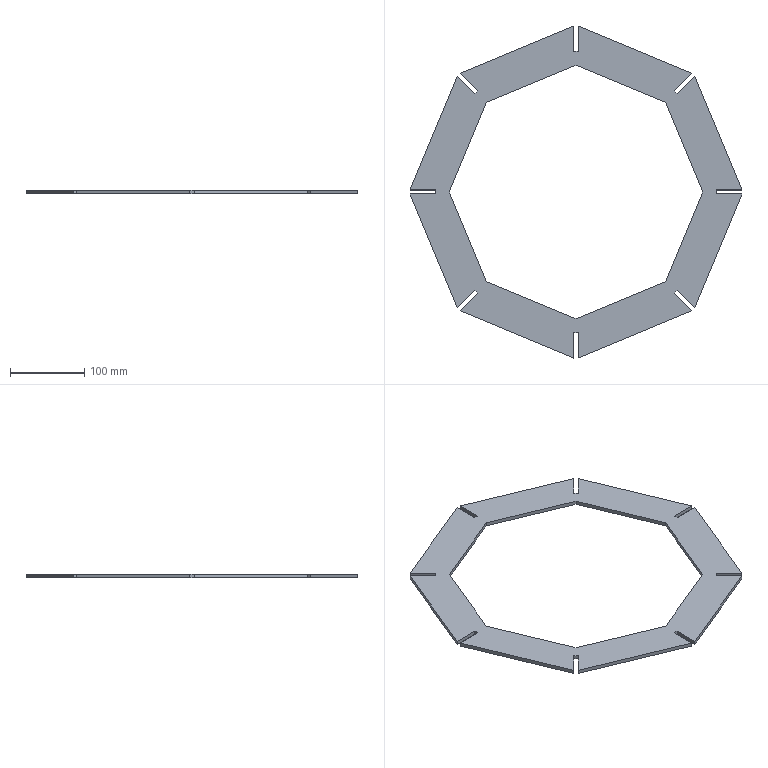Part | SolidWorks | features ICE 2, Extrusion 1 | 1 solid | 42 faces | box 447.763 x 447.763 x 5 mm | volume 295555 mm3 | plane 42
STEP:
#1=CARTESIAN_POINT('',(-2.7,223.882,0.));
#2=VERTEX_POINT('',#1);
#3=CARTESIAN_POINT('',(-156.399,160.217,0.));
#4=VERTEX_POINT('',#3);
#5=CARTESIAN_POINT('',(0.,225.,0.));
#6=DIRECTION('',(-0.9239,-0.3827,0.));
#7=VECTOR('',#6,1000.);
#8=LINE('',#5,#7);
#9=EDGE_CURVE('',#2,#4,#8,.T.);
#10=ORIENTED_EDGE('',*,*,#9,.T.);
#11=CARTESIAN_POINT('',(-156.399,160.217,5.));
#12=VERTEX_POINT('',#11);
#13=CARTESIAN_POINT('',(-156.399,160.217,5.));
#14=DIRECTION('',(0.,0.,1.));
#15=VECTOR('',#14,1000.);
#16=LINE('',#13,#15);
#17=EDGE_CURVE('',#4,#12,#16,.T.);
#18=ORIENTED_EDGE('',*,*,#17,.T.);
#19=CARTESIAN_POINT('',(-2.7,223.882,5.));
#20=VERTEX_POINT('',#19);
#21=CARTESIAN_POINT('',(0.,225.,5.));
#22=DIRECTION('',(-0.9239,-0.3827,0.));
#23=VECTOR('',#22,1000.);
#24=LINE('',#21,#23);
#25=EDGE_CURVE('',#20,#12,#24,.T.);
#26=ORIENTED_EDGE('',*,*,#25,.F.);
#27=CARTESIAN_POINT('',(-2.7,223.882,5.));
#28=DIRECTION('',(0.,0.,-1.));
#29=VECTOR('',#28,1000.);
#30=LINE('',#27,#29);
#31=EDGE_CURVE('',#20,#2,#30,.T.);
#32=ORIENTED_EDGE('',*,*,#31,.T.);
#33=EDGE_LOOP('',(#10,#18,#26,#32));
#34=FACE_OUTER_BOUND('',#33,.T.);
#35=CARTESIAN_POINT('',(0.,225.,5.));
#36=DIRECTION('',(0.3827,-0.9239,0.));
#37=DIRECTION('',(0.9239,0.3827,0.));
#38=AXIS2_PLACEMENT_3D('',#35,#36,#37);
#39=PLANE('',#38);
#40=ADVANCED_FACE('',(#34),#39,.F.);
#41=CARTESIAN_POINT('',(-160.217,156.399,0.));
#42=VERTEX_POINT('',#41);
#43=CARTESIAN_POINT('',(-223.882,2.7,0.));
#44=VERTEX_POINT('',#43);
#45=CARTESIAN_POINT('',(-159.099,159.099,0.));
#46=DIRECTION('',(-0.3827,-0.9239,0.));
#47=VECTOR('',#46,1000.);
#48=LINE('',#45,#47);
#49=EDGE_CURVE('',#42,#44,#48,.T.);
#50=ORIENTED_EDGE('',*,*,#49,.T.);
#51=CARTESIAN_POINT('',(-223.882,2.7,5.));
#52=VERTEX_POINT('',#51);
#53=CARTESIAN_POINT('',(-223.882,2.7,5.));
#54=DIRECTION('',(0.,0.,1.));
#55=VECTOR('',#54,1000.);
#56=LINE('',#53,#55);
#57=EDGE_CURVE('',#44,#52,#56,.T.);
#58=ORIENTED_EDGE('',*,*,#57,.T.);
#59=CARTESIAN_POINT('',(-160.217,156.399,5.));
#60=VERTEX_POINT('',#59);
#61=CARTESIAN_POINT('',(-159.099,159.099,5.));
#62=DIRECTION('',(-0.3827,-0.9239,0.));
#63=VECTOR('',#62,1000.);
#64=LINE('',#61,#63);
#65=EDGE_CURVE('',#60,#52,#64,.T.);
#66=ORIENTED_EDGE('',*,*,#65,.F.);
#67=CARTESIAN_POINT('',(-160.217,156.399,5.));
#68=DIRECTION('',(0.,0.,-1.));
#69=VECTOR('',#68,1000.);
#70=LINE('',#67,#69);
#71=EDGE_CURVE('',#60,#42,#70,.T.);
#72=ORIENTED_EDGE('',*,*,#71,.T.);
#73=EDGE_LOOP('',(#50,#58,#66,#72));
#74=FACE_OUTER_BOUND('',#73,.T.);
#75=CARTESIAN_POINT('',(-159.099,159.099,5.));
#76=DIRECTION('',(0.9239,-0.3827,0.));
#77=DIRECTION('',(0.3827,0.9239,0.));
#78=AXIS2_PLACEMENT_3D('',#75,#76,#77);
#79=PLANE('',#78);
#80=ADVANCED_FACE('',(#74),#79,.F.);
#81=CARTESIAN_POINT('',(-223.882,-2.7,0.));
#82=VERTEX_POINT('',#81);
#83=CARTESIAN_POINT('',(-160.217,-156.399,0.));
#84=VERTEX_POINT('',#83);
#85=CARTESIAN_POINT('',(-225.,0.,0.));
#86=DIRECTION('',(0.3827,-0.9239,0.));
#87=VECTOR('',#86,1000.);
#88=LINE('',#85,#87);
#89=EDGE_CURVE('',#82,#84,#88,.T.);
#90=ORIENTED_EDGE('',*,*,#89,.T.);
#91=CARTESIAN_POINT('',(-160.217,-156.399,5.));
#92=VERTEX_POINT('',#91);
#93=CARTESIAN_POINT('',(-160.217,-156.399,5.));
#94=DIRECTION('',(0.,0.,1.));
#95=VECTOR('',#94,1000.);
#96=LINE('',#93,#95);
#97=EDGE_CURVE('',#84,#92,#96,.T.);
#98=ORIENTED_EDGE('',*,*,#97,.T.);
#99=CARTESIAN_POINT('',(-223.882,-2.7,5.));
#100=VERTEX_POINT('',#99);
#101=CARTESIAN_POINT('',(-225.,0.,5.));
#102=DIRECTION('',(0.3827,-0.9239,0.));
#103=VECTOR('',#102,1000.);
#104=LINE('',#101,#103);
#105=EDGE_CURVE('',#100,#92,#104,.T.);
#106=ORIENTED_EDGE('',*,*,#105,.F.);
#107=CARTESIAN_POINT('',(-223.882,-2.7,5.));
#108=DIRECTION('',(0.,0.,-1.));
#109=VECTOR('',#108,1000.);
#110=LINE('',#107,#109);
#111=EDGE_CURVE('',#100,#82,#110,.T.);
#112=ORIENTED_EDGE('',*,*,#111,.T.);
#113=EDGE_LOOP('',(#90,#98,#106,#112));
#114=FACE_OUTER_BOUND('',#113,.T.);
#115=CARTESIAN_POINT('',(-225.,0.,5.));
#116=DIRECTION('',(0.9239,0.3827,0.));
#117=DIRECTION('',(-0.3827,0.9239,0.));
#118=AXIS2_PLACEMENT_3D('',#115,#116,#117);
#119=PLANE('',#118);
#120=ADVANCED_FACE('',(#114),#119,.F.);
#121=CARTESIAN_POINT('',(-156.399,-160.217,0.));
#122=VERTEX_POINT('',#121);
#123=CARTESIAN_POINT('',(-2.7,-223.882,0.));
#124=VERTEX_POINT('',#123);
#125=CARTESIAN_POINT('',(-159.099,-159.099,0.));
#126=DIRECTION('',(0.9239,-0.3827,0.));
#127=VECTOR('',#126,1000.);
#128=LINE('',#125,#127);
#129=EDGE_CURVE('',#122,#124,#128,.T.);
#130=ORIENTED_EDGE('',*,*,#129,.T.);
#131=CARTESIAN_POINT('',(-2.7,-223.882,5.));
#132=VERTEX_POINT('',#131);
#133=CARTESIAN_POINT('',(-2.7,-223.882,5.));
#134=DIRECTION('',(0.,0.,1.));
#135=VECTOR('',#134,1000.);
#136=LINE('',#133,#135);
#137=EDGE_CURVE('',#124,#132,#136,.T.);
#138=ORIENTED_EDGE('',*,*,#137,.T.);
#139=CARTESIAN_POINT('',(-156.399,-160.217,5.));
#140=VERTEX_POINT('',#139);
#141=CARTESIAN_POINT('',(-159.099,-159.099,5.));
#142=DIRECTION('',(0.9239,-0.3827,0.));
#143=VECTOR('',#142,1000.);
#144=LINE('',#141,#143);
#145=EDGE_CURVE('',#140,#132,#144,.T.);
#146=ORIENTED_EDGE('',*,*,#145,.F.);
#147=CARTESIAN_POINT('',(-156.399,-160.217,5.));
#148=DIRECTION('',(0.,0.,-1.));
#149=VECTOR('',#148,1000.);
#150=LINE('',#147,#149);
#151=EDGE_CURVE('',#140,#122,#150,.T.);
#152=ORIENTED_EDGE('',*,*,#151,.T.);
#153=EDGE_LOOP('',(#130,#138,#146,#152));
#154=FACE_OUTER_BOUND('',#153,.T.);
#155=CARTESIAN_POINT('',(-159.099,-159.099,5.));
#156=DIRECTION('',(0.3827,0.9239,0.));
#157=DIRECTION('',(-0.9239,0.3827,0.));
#158=AXIS2_PLACEMENT_3D('',#155,#156,#157);
#159=PLANE('',#158);
#160=ADVANCED_FACE('',(#154),#159,.F.);
#161=CARTESIAN_POINT('',(2.7,-223.882,0.));
#162=VERTEX_POINT('',#161);
#163=CARTESIAN_POINT('',(156.399,-160.217,0.));
#164=VERTEX_POINT('',#163);
#165=CARTESIAN_POINT('',(0.,-225.,0.));
#166=DIRECTION('',(0.9239,0.3827,0.));
#167=VECTOR('',#166,1000.);
#168=LINE('',#165,#167);
#169=EDGE_CURVE('',#162,#164,#168,.T.);
#170=ORIENTED_EDGE('',*,*,#169,.T.);
#171=CARTESIAN_POINT('',(156.399,-160.217,5.));
#172=VERTEX_POINT('',#171);
#173=CARTESIAN_POINT('',(156.399,-160.217,5.));
#174=DIRECTION('',(0.,0.,1.));
#175=VECTOR('',#174,1000.);
#176=LINE('',#173,#175);
#177=EDGE_CURVE('',#164,#172,#176,.T.);
#178=ORIENTED_EDGE('',*,*,#177,.T.);
#179=CARTESIAN_POINT('',(2.7,-223.882,5.));
#180=VERTEX_POINT('',#179);
#181=CARTESIAN_POINT('',(0.,-225.,5.));
#182=DIRECTION('',(0.9239,0.3827,0.));
#183=VECTOR('',#182,1000.);
#184=LINE('',#181,#183);
#185=EDGE_CURVE('',#180,#172,#184,.T.);
#186=ORIENTED_EDGE('',*,*,#185,.F.);
#187=CARTESIAN_POINT('',(2.7,-223.882,5.));
#188=DIRECTION('',(0.,0.,-1.));
#189=VECTOR('',#188,1000.);
#190=LINE('',#187,#189);
#191=EDGE_CURVE('',#180,#162,#190,.T.);
#192=ORIENTED_EDGE('',*,*,#191,.T.);
#193=EDGE_LOOP('',(#170,#178,#186,#192));
#194=FACE_OUTER_BOUND('',#193,.T.);
#195=CARTESIAN_POINT('',(0.,-225.,5.));
#196=DIRECTION('',(-0.3827,0.9239,0.));
#197=DIRECTION('',(-0.9239,-0.3827,0.));
#198=AXIS2_PLACEMENT_3D('',#195,#196,#197);
#199=PLANE('',#198);
#200=ADVANCED_FACE('',(#194),#199,.F.);
#201=CARTESIAN_POINT('',(160.217,-156.399,0.));
#202=VERTEX_POINT('',#201);
#203=CARTESIAN_POINT('',(223.882,-2.7,0.));
#204=VERTEX_POINT('',#203);
#205=CARTESIAN_POINT('',(159.099,-159.099,0.));
#206=DIRECTION('',(0.3827,0.9239,0.));
#207=VECTOR('',#206,1000.);
#208=LINE('',#205,#207);
#209=EDGE_CURVE('',#202,#204,#208,.T.);
#210=ORIENTED_EDGE('',*,*,#209,.T.);
#211=CARTESIAN_POINT('',(223.882,-2.7,5.));
#212=VERTEX_POINT('',#211);
#213=CARTESIAN_POINT('',(223.882,-2.7,5.));
#214=DIRECTION('',(0.,0.,1.));
#215=VECTOR('',#214,1000.);
#216=LINE('',#213,#215);
#217=EDGE_CURVE('',#204,#212,#216,.T.);
#218=ORIENTED_EDGE('',*,*,#217,.T.);
#219=CARTESIAN_POINT('',(160.217,-156.399,5.));
#220=VERTEX_POINT('',#219);
#221=CARTESIAN_POINT('',(159.099,-159.099,5.));
#222=DIRECTION('',(0.3827,0.9239,0.));
#223=VECTOR('',#222,1000.);
#224=LINE('',#221,#223);
#225=EDGE_CURVE('',#220,#212,#224,.T.);
#226=ORIENTED_EDGE('',*,*,#225,.F.);
#227=CARTESIAN_POINT('',(160.217,-156.399,5.));
#228=DIRECTION('',(0.,0.,-1.));
#229=VECTOR('',#228,1000.);
#230=LINE('',#227,#229);
#231=EDGE_CURVE('',#220,#202,#230,.T.);
#232=ORIENTED_EDGE('',*,*,#231,.T.);
#233=EDGE_LOOP('',(#210,#218,#226,#232));
#234=FACE_OUTER_BOUND('',#233,.T.);
#235=CARTESIAN_POINT('',(159.099,-159.099,5.));
#236=DIRECTION('',(-0.9239,0.3827,0.));
#237=DIRECTION('',(-0.3827,-0.9239,0.));
#238=AXIS2_PLACEMENT_3D('',#235,#236,#237);
#239=PLANE('',#238);
#240=ADVANCED_FACE('',(#234),#239,.F.);
#241=CARTESIAN_POINT('',(223.882,2.7,5.));
#242=VERTEX_POINT('',#241);
#243=CARTESIAN_POINT('',(160.217,156.399,5.));
#244=VERTEX_POINT('',#243);
#245=CARTESIAN_POINT('',(225.,0.,5.));
#246=DIRECTION('',(-0.3827,0.9239,0.));
#247=VECTOR('',#246,1000.);
#248=LINE('',#245,#247);
#249=EDGE_CURVE('',#242,#244,#248,.T.);
#250=ORIENTED_EDGE('',*,*,#249,.F.);
#251=CARTESIAN_POINT('',(223.882,2.7,0.));
#252=VERTEX_POINT('',#251);
#253=CARTESIAN_POINT('',(223.882,2.7,5.));
#254=DIRECTION('',(0.,0.,-1.));
#255=VECTOR('',#254,1000.);
#256=LINE('',#253,#255);
#257=EDGE_CURVE('',#242,#252,#256,.T.);
#258=ORIENTED_EDGE('',*,*,#257,.T.);
#259=CARTESIAN_POINT('',(160.217,156.399,0.));
#260=VERTEX_POINT('',#259);
#261=CARTESIAN_POINT('',(225.,0.,0.));
#262=DIRECTION('',(-0.3827,0.9239,0.));
#263=VECTOR('',#262,1000.);
#264=LINE('',#261,#263);
#265=EDGE_CURVE('',#252,#260,#264,.T.);
#266=ORIENTED_EDGE('',*,*,#265,.T.);
#267=CARTESIAN_POINT('',(160.217,156.399,5.));
#268=DIRECTION('',(0.,0.,1.));
#269=VECTOR('',#268,1000.);
#270=LINE('',#267,#269);
#271=EDGE_CURVE('',#260,#244,#270,.T.);
#272=ORIENTED_EDGE('',*,*,#271,.T.);
#273=EDGE_LOOP('',(#250,#258,#266,#272));
#274=FACE_OUTER_BOUND('',#273,.T.);
#275=CARTESIAN_POINT('',(225.,0.,5.));
#276=DIRECTION('',(-0.9239,-0.3827,0.));
#277=DIRECTION('',(0.3827,-0.9239,0.));
#278=AXIS2_PLACEMENT_3D('',#275,#276,#277);
#279=PLANE('',#278);
#280=ADVANCED_FACE('',(#274),#279,.F.);
#281=CARTESIAN_POINT('',(156.399,160.217,0.));
#282=VERTEX_POINT('',#281);
#283=CARTESIAN_POINT('',(2.7,223.882,0.));
#284=VERTEX_POINT('',#283);
#285=CARTESIAN_POINT('',(159.099,159.099,0.));
#286=DIRECTION('',(-0.9239,0.3827,0.));
#287=VECTOR('',#286,1000.);
#288=LINE('',#285,#287);
#289=EDGE_CURVE('',#282,#284,#288,.T.);
#290=ORIENTED_EDGE('',*,*,#289,.T.);
#291=CARTESIAN_POINT('',(2.7,223.882,5.));
#292=VERTEX_POINT('',#291);
#293=CARTESIAN_POINT('',(2.7,223.882,5.));
#294=DIRECTION('',(0.,0.,1.));
#295=VECTOR('',#294,1000.);
#296=LINE('',#293,#295);
#297=EDGE_CURVE('',#284,#292,#296,.T.);
#298=ORIENTED_EDGE('',*,*,#297,.T.);
#299=CARTESIAN_POINT('',(156.399,160.217,5.));
#300=VERTEX_POINT('',#299);
#301=CARTESIAN_POINT('',(159.099,159.099,5.));
#302=DIRECTION('',(-0.9239,0.3827,0.));
#303=VECTOR('',#302,1000.);
#304=LINE('',#301,#303);
#305=EDGE_CURVE('',#300,#292,#304,.T.);
#306=ORIENTED_EDGE('',*,*,#305,.F.);
#307=CARTESIAN_POINT('',(156.399,160.217,5.));
#308=DIRECTION('',(0.,0.,-1.));
#309=VECTOR('',#308,1000.);
#310=LINE('',#307,#309);
#311=EDGE_CURVE('',#300,#282,#310,.T.);
#312=ORIENTED_EDGE('',*,*,#311,.T.);
#313=EDGE_LOOP('',(#290,#298,#306,#312));
#314=FACE_OUTER_BOUND('',#313,.T.);
#315=CARTESIAN_POINT('',(159.099,159.099,5.));
#316=DIRECTION('',(-0.3827,-0.9239,0.));
#317=DIRECTION('',(0.9239,-0.3827,0.));
#318=AXIS2_PLACEMENT_3D('',#315,#316,#317);
#319=PLANE('',#318);
#320=ADVANCED_FACE('',(#314),#319,.F.);
#321=CARTESIAN_POINT('',(190.,2.7,5.));
#322=VERTEX_POINT('',#321);
#323=CARTESIAN_POINT('',(260.,2.7,5.));
#324=DIRECTION('',(-1.,0.,0.));
#325=VECTOR('',#324,1000.);
#326=LINE('',#323,#325);
#327=EDGE_CURVE('',#242,#322,#326,.T.);
#328=ORIENTED_EDGE('',*,*,#327,.F.);
#329=ORIENTED_EDGE('',*,*,#249,.T.);
#330=CARTESIAN_POINT('',(136.259,132.441,5.));
#331=VERTEX_POINT('',#330);
#332=CARTESIAN_POINT('',(185.757,181.939,5.));
#333=DIRECTION('',(0.7071,0.7071,0.));
#334=VECTOR('',#333,1000.);
#335=LINE('',#332,#334);
#336=EDGE_CURVE('',#331,#244,#335,.T.);
#337=ORIENTED_EDGE('',*,*,#336,.F.);
#338=CARTESIAN_POINT('',(132.441,136.259,5.));
#339=VERTEX_POINT('',#338);
#340=CARTESIAN_POINT('',(136.259,132.441,5.));
#341=DIRECTION('',(0.7071,-0.7071,0.));
#342=VECTOR('',#341,1000.);
#343=LINE('',#340,#342);
#344=EDGE_CURVE('',#339,#331,#343,.T.);
#345=ORIENTED_EDGE('',*,*,#344,.F.);
#346=CARTESIAN_POINT('',(181.939,185.757,5.));
#347=DIRECTION('',(-0.7071,-0.7071,0.));
#348=VECTOR('',#347,1000.);
#349=LINE('',#346,#348);
#350=EDGE_CURVE('',#300,#339,#349,.T.);
#351=ORIENTED_EDGE('',*,*,#350,.F.);
#352=ORIENTED_EDGE('',*,*,#305,.T.);
#353=CARTESIAN_POINT('',(2.7,190.,5.));
#354=VERTEX_POINT('',#353);
#355=CARTESIAN_POINT('',(2.7,260.,5.));
#356=DIRECTION('',(0.,1.,0.));
#357=VECTOR('',#356,1000.);
#358=LINE('',#355,#357);
#359=EDGE_CURVE('',#354,#292,#358,.T.);
#360=ORIENTED_EDGE('',*,*,#359,.F.);
#361=CARTESIAN_POINT('',(-2.7,190.,5.));
#362=VERTEX_POINT('',#361);
#363=CARTESIAN_POINT('',(2.7,190.,5.));
#364=DIRECTION('',(1.,0.,0.));
#365=VECTOR('',#364,1000.);
#366=LINE('',#363,#365);
#367=EDGE_CURVE('',#362,#354,#366,.T.);
#368=ORIENTED_EDGE('',*,*,#367,.F.);
#369=CARTESIAN_POINT('',(-2.7,260.,5.));
#370=DIRECTION('',(0.,-1.,0.));
#371=VECTOR('',#370,1000.);
#372=LINE('',#369,#371);
#373=EDGE_CURVE('',#20,#362,#372,.T.);
#374=ORIENTED_EDGE('',*,*,#373,.F.);
#375=ORIENTED_EDGE('',*,*,#25,.T.);
#376=CARTESIAN_POINT('',(-132.441,136.259,5.));
#377=VERTEX_POINT('',#376);
#378=CARTESIAN_POINT('',(-181.939,185.757,5.));
#379=DIRECTION('',(-0.7071,0.7071,0.));
#380=VECTOR('',#379,1000.);
#381=LINE('',#378,#380);
#382=EDGE_CURVE('',#377,#12,#381,.T.);
#383=ORIENTED_EDGE('',*,*,#382,.F.);
#384=CARTESIAN_POINT('',(-136.259,132.441,5.));
#385=VERTEX_POINT('',#384);
#386=CARTESIAN_POINT('',(-132.441,136.259,5.));
#387=DIRECTION('',(0.7071,0.7071,0.));
#388=VECTOR('',#387,1000.);
#389=LINE('',#386,#388);
#390=EDGE_CURVE('',#385,#377,#389,.T.);
#391=ORIENTED_EDGE('',*,*,#390,.F.);
#392=CARTESIAN_POINT('',(-185.757,181.939,5.));
#393=DIRECTION('',(0.7071,-0.7071,0.));
#394=VECTOR('',#393,1000.);
#395=LINE('',#392,#394);
#396=EDGE_CURVE('',#60,#385,#395,.T.);
#397=ORIENTED_EDGE('',*,*,#396,.F.);
#398=ORIENTED_EDGE('',*,*,#65,.T.);
#399=CARTESIAN_POINT('',(-190.,2.7,5.));
#400=VERTEX_POINT('',#399);
#401=CARTESIAN_POINT('',(-260.,2.7,5.));
#402=DIRECTION('',(-1.,0.,0.));
#403=VECTOR('',#402,1000.);
#404=LINE('',#401,#403);
#405=EDGE_CURVE('',#400,#52,#404,.T.);
#406=ORIENTED_EDGE('',*,*,#405,.F.);
#407=CARTESIAN_POINT('',(-190.,-2.7,5.));
#408=VERTEX_POINT('',#407);
#409=CARTESIAN_POINT('',(-190.,2.7,5.));
#410=DIRECTION('',(0.,1.,0.));
#411=VECTOR('',#410,1000.);
#412=LINE('',#409,#411);
#413=EDGE_CURVE('',#408,#400,#412,.T.);
#414=ORIENTED_EDGE('',*,*,#413,.F.);
#415=CARTESIAN_POINT('',(-260.,-2.7,5.));
#416=DIRECTION('',(1.,0.,0.));
#417=VECTOR('',#416,1000.);
#418=LINE('',#415,#417);
#419=EDGE_CURVE('',#100,#408,#418,.T.);
#420=ORIENTED_EDGE('',*,*,#419,.F.);
#421=ORIENTED_EDGE('',*,*,#105,.T.);
#422=CARTESIAN_POINT('',(-136.259,-132.441,5.));
#423=VERTEX_POINT('',#422);
#424=CARTESIAN_POINT('',(-185.757,-181.939,5.));
#425=DIRECTION('',(-0.7071,-0.7071,0.));
#426=VECTOR('',#425,1000.);
#427=LINE('',#424,#426);
#428=EDGE_CURVE('',#423,#92,#427,.T.);
#429=ORIENTED_EDGE('',*,*,#428,.F.);
#430=CARTESIAN_POINT('',(-132.441,-136.259,5.));
#431=VERTEX_POINT('',#430);
#432=CARTESIAN_POINT('',(-136.259,-132.441,5.));
#433=DIRECTION('',(-0.7071,0.7071,0.));
#434=VECTOR('',#433,1000.);
#435=LINE('',#432,#434);
#436=EDGE_CURVE('',#431,#423,#435,.T.);
#437=ORIENTED_EDGE('',*,*,#436,.F.);
#438=CARTESIAN_POINT('',(-181.939,-185.757,5.));
#439=DIRECTION('',(0.7071,0.7071,0.));
#440=VECTOR('',#439,1000.);
#441=LINE('',#438,#440);
#442=EDGE_CURVE('',#140,#431,#441,.T.);
#443=ORIENTED_EDGE('',*,*,#442,.F.);
#444=ORIENTED_EDGE('',*,*,#145,.T.);
#445=CARTESIAN_POINT('',(-2.7,-190.,5.));
#446=VERTEX_POINT('',#445);
#447=CARTESIAN_POINT('',(-2.7,-260.,5.));
#448=DIRECTION('',(0.,-1.,0.));
#449=VECTOR('',#448,1000.);
#450=LINE('',#447,#449);
#451=EDGE_CURVE('',#446,#132,#450,.T.);
#452=ORIENTED_EDGE('',*,*,#451,.F.);
#453=CARTESIAN_POINT('',(2.7,-190.,5.));
#454=VERTEX_POINT('',#453);
#455=CARTESIAN_POINT('',(-2.7,-190.,5.));
#456=DIRECTION('',(-1.,0.,0.));
#457=VECTOR('',#456,1000.);
#458=LINE('',#455,#457);
#459=EDGE_CURVE('',#454,#446,#458,.T.);
#460=ORIENTED_EDGE('',*,*,#459,.F.);
#461=CARTESIAN_POINT('',(2.7,-260.,5.));
#462=DIRECTION('',(0.,1.,0.));
#463=VECTOR('',#462,1000.);
#464=LINE('',#461,#463);
#465=EDGE_CURVE('',#180,#454,#464,.T.);
#466=ORIENTED_EDGE('',*,*,#465,.F.);
#467=ORIENTED_EDGE('',*,*,#185,.T.);
#468=CARTESIAN_POINT('',(132.441,-136.259,5.));
#469=VERTEX_POINT('',#468);
#470=CARTESIAN_POINT('',(181.939,-185.757,5.));
#471=DIRECTION('',(0.7071,-0.7071,0.));
#472=VECTOR('',#471,1000.);
#473=LINE('',#470,#472);
#474=EDGE_CURVE('',#469,#172,#473,.T.);
#475=ORIENTED_EDGE('',*,*,#474,.F.);
#476=CARTESIAN_POINT('',(136.259,-132.441,5.));
#477=VERTEX_POINT('',#476);
#478=CARTESIAN_POINT('',(132.441,-136.259,5.));
#479=DIRECTION('',(-0.7071,-0.7071,0.));
#480=VECTOR('',#479,1000.);
#481=LINE('',#478,#480);
#482=EDGE_CURVE('',#477,#469,#481,.T.);
#483=ORIENTED_EDGE('',*,*,#482,.F.);
#484=CARTESIAN_POINT('',(185.757,-181.939,5.));
#485=DIRECTION('',(-0.7071,0.7071,0.));
#486=VECTOR('',#485,1000.);
#487=LINE('',#484,#486);
#488=EDGE_CURVE('',#220,#477,#487,.T.);
#489=ORIENTED_EDGE('',*,*,#488,.F.);
#490=ORIENTED_EDGE('',*,*,#225,.T.);
#491=CARTESIAN_POINT('',(190.,-2.7,5.));
#492=VERTEX_POINT('',#491);
#493=CARTESIAN_POINT('',(260.,-2.7,5.));
#494=DIRECTION('',(1.,0.,0.));
#495=VECTOR('',#494,1000.);
#496=LINE('',#493,#495);
#497=EDGE_CURVE('',#492,#212,#496,.T.);
#498=ORIENTED_EDGE('',*,*,#497,.F.);
#499=CARTESIAN_POINT('',(190.,-2.7,5.));
#500=DIRECTION('',(0.,-1.,0.));
#501=VECTOR('',#500,1000.);
#502=LINE('',#499,#501);
#503=EDGE_CURVE('',#322,#492,#502,.T.);
#504=ORIENTED_EDGE('',*,*,#503,.F.);
#505=EDGE_LOOP('',(#328,#329,#337,#345,#351,#352,#360,#368,#374,#375,#383,#391,#397,#398,#406,#414,#420,#421,#429,#437,#443,#444,#452,#460,#466,#467,#475,#483,#489,#490,#498,#504));
#506=FACE_OUTER_BOUND('',#505,.T.);
#507=CARTESIAN_POINT('',(120.831,120.831,5.));
#508=VERTEX_POINT('',#507);
#509=CARTESIAN_POINT('',(0.,170.88,5.));
#510=VERTEX_POINT('',#509);
#511=CARTESIAN_POINT('',(120.831,120.831,5.));
#512=DIRECTION('',(-0.9239,0.3827,0.));
#513=VECTOR('',#512,1000.);
#514=LINE('',#511,#513);
#515=EDGE_CURVE('',#508,#510,#514,.T.);
#516=ORIENTED_EDGE('',*,*,#515,.F.);
#517=CARTESIAN_POINT('',(170.88,0.,5.));
#518=VERTEX_POINT('',#517);
#519=CARTESIAN_POINT('',(170.88,0.,5.));
#520=DIRECTION('',(-0.3827,0.9239,0.));
#521=VECTOR('',#520,1000.);
#522=LINE('',#519,#521);
#523=EDGE_CURVE('',#518,#508,#522,.T.);
#524=ORIENTED_EDGE('',*,*,#523,.F.);
#525=CARTESIAN_POINT('',(120.831,-120.831,5.));
#526=VERTEX_POINT('',#525);
#527=CARTESIAN_POINT('',(120.831,-120.831,5.));
#528=DIRECTION('',(0.3827,0.9239,0.));
#529=VECTOR('',#528,1000.);
#530=LINE('',#527,#529);
#531=EDGE_CURVE('',#526,#518,#530,.T.);
#532=ORIENTED_EDGE('',*,*,#531,.F.);
#533=CARTESIAN_POINT('',(0.,-170.88,5.));
#534=VERTEX_POINT('',#533);
#535=CARTESIAN_POINT('',(0.,-170.88,5.));
#536=DIRECTION('',(0.9239,0.3827,0.));
#537=VECTOR('',#536,1000.);
#538=LINE('',#535,#537);
#539=EDGE_CURVE('',#534,#526,#538,.T.);
#540=ORIENTED_EDGE('',*,*,#539,.F.);
#541=CARTESIAN_POINT('',(-120.831,-120.831,5.));
#542=VERTEX_POINT('',#541);
#543=CARTESIAN_POINT('',(-120.831,-120.831,5.));
#544=DIRECTION('',(0.9239,-0.3827,0.));
#545=VECTOR('',#544,1000.);
#546=LINE('',#543,#545);
#547=EDGE_CURVE('',#542,#534,#546,.T.);
#548=ORIENTED_EDGE('',*,*,#547,.F.);
#549=CARTESIAN_POINT('',(-170.88,0.,5.));
#550=VERTEX_POINT('',#549);
#551=CARTESIAN_POINT('',(-170.88,0.,5.));
#552=DIRECTION('',(0.3827,-0.9239,0.));
#553=VECTOR('',#552,1000.);
#554=LINE('',#551,#553);
#555=EDGE_CURVE('',#550,#542,#554,.T.);
#556=ORIENTED_EDGE('',*,*,#555,.F.);
#557=CARTESIAN_POINT('',(-120.831,120.831,5.));
#558=VERTEX_POINT('',#557);
#559=CARTESIAN_POINT('',(-120.831,120.831,5.));
#560=DIRECTION('',(-0.3827,-0.9239,0.));
#561=VECTOR('',#560,1000.);
#562=LINE('',#559,#561);
#563=EDGE_CURVE('',#558,#550,#562,.T.);
#564=ORIENTED_EDGE('',*,*,#563,.F.);
#565=CARTESIAN_POINT('',(0.,170.88,5.));
#566=DIRECTION('',(-0.9239,-0.3827,0.));
#567=VECTOR('',#566,1000.);
#568=LINE('',#565,#567);
#569=EDGE_CURVE('',#510,#558,#568,.T.);
#570=ORIENTED_EDGE('',*,*,#569,.F.);
#571=EDGE_LOOP('',(#516,#524,#532,#540,#548,#556,#564,#570));
#572=FACE_BOUND('',#571,.T.);
#573=CARTESIAN_POINT('',(0.,0.,5.));
#574=DIRECTION('',(0.,0.,1.));
#575=DIRECTION('',(1.,0.,0.));
#576=AXIS2_PLACEMENT_3D('',#573,#574,#575);
#577=PLANE('',#576);
#578=ADVANCED_FACE('',(#506,#572),#577,.T.);
#579=CARTESIAN_POINT('',(170.88,0.,0.));
#580=VERTEX_POINT('',#579);
#581=CARTESIAN_POINT('',(120.831,120.831,0.));
#582=VERTEX_POINT('',#581);
#583=CARTESIAN_POINT('',(145.856,60.415,0.));
#584=DIRECTION('',(-0.3827,0.9239,0.));
#585=VECTOR('',#584,1000.);
#586=LINE('',#583,#585);
#587=EDGE_CURVE('',#580,#582,#586,.T.);
#588=ORIENTED_EDGE('',*,*,#587,.T.);
#589=CARTESIAN_POINT('',(0.,170.88,0.));
#590=VERTEX_POINT('',#589);
#591=CARTESIAN_POINT('',(60.415,145.856,0.));
#592=DIRECTION('',(-0.9239,0.3827,0.));
#593=VECTOR('',#592,1000.);
#594=LINE('',#591,#593);
#595=EDGE_CURVE('',#582,#590,#594,.T.);
#596=ORIENTED_EDGE('',*,*,#595,.T.);
#597=CARTESIAN_POINT('',(-120.831,120.831,0.));
#598=VERTEX_POINT('',#597);
#599=CARTESIAN_POINT('',(-60.415,145.856,0.));
#600=DIRECTION('',(-0.9239,-0.3827,0.));
#601=VECTOR('',#600,1000.);
#602=LINE('',#599,#601);
#603=EDGE_CURVE('',#590,#598,#602,.T.);
#604=ORIENTED_EDGE('',*,*,#603,.T.);
#605=CARTESIAN_POINT('',(-170.88,0.,0.));
#606=VERTEX_POINT('',#605);
#607=CARTESIAN_POINT('',(-145.856,60.415,0.));
#608=DIRECTION('',(-0.3827,-0.9239,0.));
#609=VECTOR('',#608,1000.);
#610=LINE('',#607,#609);
#611=EDGE_CURVE('',#598,#606,#610,.T.);
#612=ORIENTED_EDGE('',*,*,#611,.T.);
#613=CARTESIAN_POINT('',(-120.831,-120.831,0.));
#614=VERTEX_POINT('',#613);
#615=CARTESIAN_POINT('',(-145.856,-60.415,0.));
#616=DIRECTION('',(0.3827,-0.9239,0.));
#617=VECTOR('',#616,1000.);
#618=LINE('',#615,#617);
#619=EDGE_CURVE('',#606,#614,#618,.T.);
#620=ORIENTED_EDGE('',*,*,#619,.T.);
#621=CARTESIAN_POINT('',(0.,-170.88,0.));
#622=VERTEX_POINT('',#621);
#623=CARTESIAN_POINT('',(-60.415,-145.856,0.));
#624=DIRECTION('',(0.9239,-0.3827,0.));
#625=VECTOR('',#624,1000.);
#626=LINE('',#623,#625);
#627=EDGE_CURVE('',#614,#622,#626,.T.);
#628=ORIENTED_EDGE('',*,*,#627,.T.);
#629=CARTESIAN_POINT('',(120.831,-120.831,0.));
#630=VERTEX_POINT('',#629);
#631=CARTESIAN_POINT('',(60.415,-145.856,0.));
#632=DIRECTION('',(0.9239,0.3827,0.));
#633=VECTOR('',#632,1000.);
#634=LINE('',#631,#633);
#635=EDGE_CURVE('',#622,#630,#634,.T.);
#636=ORIENTED_EDGE('',*,*,#635,.T.);
#637=CARTESIAN_POINT('',(145.856,-60.415,0.));
#638=DIRECTION('',(0.3827,0.9239,0.));
#639=VECTOR('',#638,1000.);
#640=LINE('',#637,#639);
#641=EDGE_CURVE('',#630,#580,#640,.T.);
#642=ORIENTED_EDGE('',*,*,#641,.T.);
#643=EDGE_LOOP('',(#588,#596,#604,#612,#620,#628,#636,#642));
#644=FACE_BOUND('',#643,.T.);
#645=ORIENTED_EDGE('',*,*,#265,.F.);
#646=CARTESIAN_POINT('',(190.,2.7,0.));
#647=VERTEX_POINT('',#646);
#648=CARTESIAN_POINT('',(0.,2.7,0.));
#649=DIRECTION('',(-1.,0.,0.));
#650=VECTOR('',#649,1000.);
#651=LINE('',#648,#650);
#652=EDGE_CURVE('',#252,#647,#651,.T.);
#653=ORIENTED_EDGE('',*,*,#652,.T.);
#654=CARTESIAN_POINT('',(190.,-2.7,0.));
#655=VERTEX_POINT('',#654);
#656=CARTESIAN_POINT('',(190.,0.,0.));
#657=DIRECTION('',(0.,-1.,0.));
#658=VECTOR('',#657,1000.);
#659=LINE('',#656,#658);
#660=EDGE_CURVE('',#647,#655,#659,.T.);
#661=ORIENTED_EDGE('',*,*,#660,.T.);
#662=CARTESIAN_POINT('',(0.,-2.7,0.));
#663=DIRECTION('',(1.,0.,0.));
#664=VECTOR('',#663,1000.);
#665=LINE('',#662,#664);
#666=EDGE_CURVE('',#655,#204,#665,.T.);
#667=ORIENTED_EDGE('',*,*,#666,.T.);
#668=ORIENTED_EDGE('',*,*,#209,.F.);
#669=CARTESIAN_POINT('',(136.259,-132.441,0.));
#670=VERTEX_POINT('',#669);
#671=CARTESIAN_POINT('',(1.909,1.909,0.));
#672=DIRECTION('',(-0.7071,0.7071,0.));
#673=VECTOR('',#672,1000.);
#674=LINE('',#671,#673);
#675=EDGE_CURVE('',#202,#670,#674,.T.);
#676=ORIENTED_EDGE('',*,*,#675,.T.);
#677=CARTESIAN_POINT('',(132.441,-136.259,0.));
#678=VERTEX_POINT('',#677);
#679=CARTESIAN_POINT('',(134.35,-134.35,0.));
#680=DIRECTION('',(-0.7071,-0.7071,0.));
#681=VECTOR('',#680,1000.);
#682=LINE('',#679,#681);
#683=EDGE_CURVE('',#670,#678,#682,.T.);
#684=ORIENTED_EDGE('',*,*,#683,.T.);
#685=CARTESIAN_POINT('',(-1.909,-1.909,0.));
#686=DIRECTION('',(0.7071,-0.7071,0.));
#687=VECTOR('',#686,1000.);
#688=LINE('',#685,#687);
#689=EDGE_CURVE('',#678,#164,#688,.T.);
#690=ORIENTED_EDGE('',*,*,#689,.T.);
#691=ORIENTED_EDGE('',*,*,#169,.F.);
#692=CARTESIAN_POINT('',(2.7,-190.,0.));
#693=VERTEX_POINT('',#692);
#694=CARTESIAN_POINT('',(2.7,0.,0.));
#695=DIRECTION('',(0.,1.,0.));
#696=VECTOR('',#695,1000.);
#697=LINE('',#694,#696);
#698=EDGE_CURVE('',#162,#693,#697,.T.);
#699=ORIENTED_EDGE('',*,*,#698,.T.);
#700=CARTESIAN_POINT('',(-2.7,-190.,0.));
#701=VERTEX_POINT('',#700);
#702=CARTESIAN_POINT('',(0.,-190.,0.));
#703=DIRECTION('',(-1.,0.,0.));
#704=VECTOR('',#703,1000.);
#705=LINE('',#702,#704);
#706=EDGE_CURVE('',#693,#701,#705,.T.);
#707=ORIENTED_EDGE('',*,*,#706,.T.);
#708=CARTESIAN_POINT('',(-2.7,0.,0.));
#709=DIRECTION('',(0.,-1.,0.));
#710=VECTOR('',#709,1000.);
#711=LINE('',#708,#710);
#712=EDGE_CURVE('',#701,#124,#711,.T.);
#713=ORIENTED_EDGE('',*,*,#712,.T.);
#714=ORIENTED_EDGE('',*,*,#129,.F.);
#715=CARTESIAN_POINT('',(-132.441,-136.259,0.));
#716=VERTEX_POINT('',#715);
#717=CARTESIAN_POINT('',(1.909,-1.909,0.));
#718=DIRECTION('',(0.7071,0.7071,0.));
#719=VECTOR('',#718,1000.);
#720=LINE('',#717,#719);
#721=EDGE_CURVE('',#122,#716,#720,.T.);
#722=ORIENTED_EDGE('',*,*,#721,.T.);
#723=CARTESIAN_POINT('',(-136.259,-132.441,0.));
#724=VERTEX_POINT('',#723);
#725=CARTESIAN_POINT('',(-134.35,-134.35,0.));
#726=DIRECTION('',(-0.7071,0.7071,0.));
#727=VECTOR('',#726,1000.);
#728=LINE('',#725,#727);
#729=EDGE_CURVE('',#716,#724,#728,.T.);
#730=ORIENTED_EDGE('',*,*,#729,.T.);
#731=CARTESIAN_POINT('',(-1.909,1.909,0.));
#732=DIRECTION('',(-0.7071,-0.7071,0.));
#733=VECTOR('',#732,1000.);
#734=LINE('',#731,#733);
#735=EDGE_CURVE('',#724,#84,#734,.T.);
#736=ORIENTED_EDGE('',*,*,#735,.T.);
#737=ORIENTED_EDGE('',*,*,#89,.F.);
#738=CARTESIAN_POINT('',(-190.,-2.7,0.));
#739=VERTEX_POINT('',#738);
#740=CARTESIAN_POINT('',(0.,-2.7,0.));
#741=DIRECTION('',(1.,0.,0.));
#742=VECTOR('',#741,1000.);
#743=LINE('',#740,#742);
#744=EDGE_CURVE('',#82,#739,#743,.T.);
#745=ORIENTED_EDGE('',*,*,#744,.T.);
#746=CARTESIAN_POINT('',(-190.,2.7,0.));
#747=VERTEX_POINT('',#746);
#748=CARTESIAN_POINT('',(-190.,0.,0.));
#749=DIRECTION('',(0.,1.,0.));
#750=VECTOR('',#749,1000.);
#751=LINE('',#748,#750);
#752=EDGE_CURVE('',#739,#747,#751,.T.);
#753=ORIENTED_EDGE('',*,*,#752,.T.);
#754=CARTESIAN_POINT('',(0.,2.7,0.));
#755=DIRECTION('',(-1.,0.,0.));
#756=VECTOR('',#755,1000.);
#757=LINE('',#754,#756);
#758=EDGE_CURVE('',#747,#44,#757,.T.);
#759=ORIENTED_EDGE('',*,*,#758,.T.);
#760=ORIENTED_EDGE('',*,*,#49,.F.);
#761=CARTESIAN_POINT('',(-136.259,132.441,0.));
#762=VERTEX_POINT('',#761);
#763=CARTESIAN_POINT('',(-1.909,-1.909,0.));
#764=DIRECTION('',(0.7071,-0.7071,0.));
#765=VECTOR('',#764,1000.);
#766=LINE('',#763,#765);
#767=EDGE_CURVE('',#42,#762,#766,.T.);
#768=ORIENTED_EDGE('',*,*,#767,.T.);
#769=CARTESIAN_POINT('',(-132.441,136.259,0.));
#770=VERTEX_POINT('',#769);
#771=CARTESIAN_POINT('',(-134.35,134.35,0.));
#772=DIRECTION('',(0.7071,0.7071,0.));
#773=VECTOR('',#772,1000.);
#774=LINE('',#771,#773);
#775=EDGE_CURVE('',#762,#770,#774,.T.);
#776=ORIENTED_EDGE('',*,*,#775,.T.);
#777=CARTESIAN_POINT('',(1.909,1.909,0.));
#778=DIRECTION('',(-0.7071,0.7071,0.));
#779=VECTOR('',#778,1000.);
#780=LINE('',#777,#779);
#781=EDGE_CURVE('',#770,#4,#780,.T.);
#782=ORIENTED_EDGE('',*,*,#781,.T.);
#783=ORIENTED_EDGE('',*,*,#9,.F.);
#784=CARTESIAN_POINT('',(-2.7,190.,0.));
#785=VERTEX_POINT('',#784);
#786=CARTESIAN_POINT('',(-2.7,0.,0.));
#787=DIRECTION('',(0.,-1.,0.));
#788=VECTOR('',#787,1000.);
#789=LINE('',#786,#788);
#790=EDGE_CURVE('',#2,#785,#789,.T.);
#791=ORIENTED_EDGE('',*,*,#790,.T.);
#792=CARTESIAN_POINT('',(2.7,190.,0.));
#793=VERTEX_POINT('',#792);
#794=CARTESIAN_POINT('',(0.,190.,0.));
#795=DIRECTION('',(1.,0.,0.));
#796=VECTOR('',#795,1000.);
#797=LINE('',#794,#796);
#798=EDGE_CURVE('',#785,#793,#797,.T.);
#799=ORIENTED_EDGE('',*,*,#798,.T.);
#800=CARTESIAN_POINT('',(2.7,0.,0.));
#801=DIRECTION('',(0.,1.,0.));
#802=VECTOR('',#801,1000.);
#803=LINE('',#800,#802);
#804=EDGE_CURVE('',#793,#284,#803,.T.);
#805=ORIENTED_EDGE('',*,*,#804,.T.);
#806=ORIENTED_EDGE('',*,*,#289,.F.);
#807=CARTESIAN_POINT('',(132.441,136.259,0.));
#808=VERTEX_POINT('',#807);
#809=CARTESIAN_POINT('',(-1.909,1.909,0.));
#810=DIRECTION('',(-0.7071,-0.7071,0.));
#811=VECTOR('',#810,1000.);
#812=LINE('',#809,#811);
#813=EDGE_CURVE('',#282,#808,#812,.T.);
#814=ORIENTED_EDGE('',*,*,#813,.T.);
#815=CARTESIAN_POINT('',(136.259,132.441,0.));
#816=VERTEX_POINT('',#815);
#817=CARTESIAN_POINT('',(134.35,134.35,0.));
#818=DIRECTION('',(0.7071,-0.7071,0.));
#819=VECTOR('',#818,1000.);
#820=LINE('',#817,#819);
#821=EDGE_CURVE('',#808,#816,#820,.T.);
#822=ORIENTED_EDGE('',*,*,#821,.T.);
#823=CARTESIAN_POINT('',(1.909,-1.909,0.));
#824=DIRECTION('',(0.7071,0.7071,0.));
#825=VECTOR('',#824,1000.);
#826=LINE('',#823,#825);
#827=EDGE_CURVE('',#816,#260,#826,.T.);
#828=ORIENTED_EDGE('',*,*,#827,.T.);
#829=EDGE_LOOP('',(#645,#653,#661,#667,#668,#676,#684,#690,#691,#699,#707,#713,#714,#722,#730,#736,#737,#745,#753,#759,#760,#768,#776,#782,#783,#791,#799,#805,#806,#814,#822,#828));
#830=FACE_OUTER_BOUND('',#829,.T.);
#831=CARTESIAN_POINT('',(0.,0.,0.));
#832=DIRECTION('',(0.,0.,1.));
#833=DIRECTION('',(1.,0.,0.));
#834=AXIS2_PLACEMENT_3D('',#831,#832,#833);
#835=PLANE('',#834);
#836=ADVANCED_FACE('',(#644,#830),#835,.F.);
#837=CARTESIAN_POINT('',(120.831,120.831,-601.));
#838=DIRECTION('',(0.,0.,1.));
#839=VECTOR('',#838,1000.);
#840=LINE('',#837,#839);
#841=EDGE_CURVE('',#582,#508,#840,.T.);
#842=ORIENTED_EDGE('',*,*,#841,.T.);
#843=ORIENTED_EDGE('',*,*,#515,.T.);
#844=CARTESIAN_POINT('',(0.,170.88,-601.));
#845=DIRECTION('',(0.,0.,1.));
#846=VECTOR('',#845,1000.);
#847=LINE('',#844,#846);
#848=EDGE_CURVE('',#590,#510,#847,.T.);
#849=ORIENTED_EDGE('',*,*,#848,.F.);
#850=ORIENTED_EDGE('',*,*,#595,.F.);
#851=EDGE_LOOP('',(#842,#843,#849,#850));
#852=FACE_OUTER_BOUND('',#851,.T.);
#853=CARTESIAN_POINT('',(120.831,120.831,-601.));
#854=DIRECTION('',(0.3827,0.9239,0.));
#855=DIRECTION('',(-0.9239,0.3827,0.));
#856=AXIS2_PLACEMENT_3D('',#853,#854,#855);
#857=PLANE('',#856);
#858=ADVANCED_FACE('',(#852),#857,.F.);
#859=CARTESIAN_POINT('',(170.88,0.,-601.));
#860=DIRECTION('',(0.,0.,1.));
#861=VECTOR('',#860,1000.);
#862=LINE('',#859,#861);
#863=EDGE_CURVE('',#580,#518,#862,.T.);
#864=ORIENTED_EDGE('',*,*,#863,.T.);
#865=ORIENTED_EDGE('',*,*,#523,.T.);
#866=ORIENTED_EDGE('',*,*,#841,.F.);
#867=ORIENTED_EDGE('',*,*,#587,.F.);
#868=EDGE_LOOP('',(#864,#865,#866,#867));
#869=FACE_OUTER_BOUND('',#868,.T.);
#870=CARTESIAN_POINT('',(170.88,0.,-601.));
#871=DIRECTION('',(0.9239,0.3827,0.));
#872=DIRECTION('',(-0.3827,0.9239,0.));
#873=AXIS2_PLACEMENT_3D('',#870,#871,#872);
#874=PLANE('',#873);
#875=ADVANCED_FACE('',(#869),#874,.F.);
#876=CARTESIAN_POINT('',(120.831,-120.831,-601.));
#877=DIRECTION('',(0.,0.,1.));
#878=VECTOR('',#877,1000.);
#879=LINE('',#876,#878);
#880=EDGE_CURVE('',#630,#526,#879,.T.);
#881=ORIENTED_EDGE('',*,*,#880,.T.);
#882=ORIENTED_EDGE('',*,*,#531,.T.);
#883=ORIENTED_EDGE('',*,*,#863,.F.);
#884=ORIENTED_EDGE('',*,*,#641,.F.);
#885=EDGE_LOOP('',(#881,#882,#883,#884));
#886=FACE_OUTER_BOUND('',#885,.T.);
#887=CARTESIAN_POINT('',(120.831,-120.831,-601.));
#888=DIRECTION('',(0.9239,-0.3827,0.));
#889=DIRECTION('',(0.3827,0.9239,0.));
#890=AXIS2_PLACEMENT_3D('',#887,#888,#889);
#891=PLANE('',#890);
#892=ADVANCED_FACE('',(#886),#891,.F.);
#893=CARTESIAN_POINT('',(0.,-170.88,-601.));
#894=DIRECTION('',(0.,0.,1.));
#895=VECTOR('',#894,1000.);
#896=LINE('',#893,#895);
#897=EDGE_CURVE('',#622,#534,#896,.T.);
#898=ORIENTED_EDGE('',*,*,#897,.T.);
#899=ORIENTED_EDGE('',*,*,#539,.T.);
#900=ORIENTED_EDGE('',*,*,#880,.F.);
#901=ORIENTED_EDGE('',*,*,#635,.F.);
#902=EDGE_LOOP('',(#898,#899,#900,#901));
#903=FACE_OUTER_BOUND('',#902,.T.);
#904=CARTESIAN_POINT('',(0.,-170.88,-601.));
#905=DIRECTION('',(0.3827,-0.9239,0.));
#906=DIRECTION('',(0.9239,0.3827,0.));
#907=AXIS2_PLACEMENT_3D('',#904,#905,#906);
#908=PLANE('',#907);
#909=ADVANCED_FACE('',(#903),#908,.F.);
#910=CARTESIAN_POINT('',(-120.831,-120.831,-601.));
#911=DIRECTION('',(0.,0.,1.));
#912=VECTOR('',#911,1000.);
#913=LINE('',#910,#912);
#914=EDGE_CURVE('',#614,#542,#913,.T.);
#915=ORIENTED_EDGE('',*,*,#914,.T.);
#916=ORIENTED_EDGE('',*,*,#547,.T.);
#917=ORIENTED_EDGE('',*,*,#897,.F.);
#918=ORIENTED_EDGE('',*,*,#627,.F.);
#919=EDGE_LOOP('',(#915,#916,#917,#918));
#920=FACE_OUTER_BOUND('',#919,.T.);
#921=CARTESIAN_POINT('',(-120.831,-120.831,-601.));
#922=DIRECTION('',(-0.3827,-0.9239,0.));
#923=DIRECTION('',(0.9239,-0.3827,0.));
#924=AXIS2_PLACEMENT_3D('',#921,#922,#923);
#925=PLANE('',#924);
#926=ADVANCED_FACE('',(#920),#925,.F.);
#927=CARTESIAN_POINT('',(-170.88,0.,-601.));
#928=DIRECTION('',(0.,0.,1.));
#929=VECTOR('',#928,1000.);
#930=LINE('',#927,#929);
#931=EDGE_CURVE('',#606,#550,#930,.T.);
#932=ORIENTED_EDGE('',*,*,#931,.T.);
#933=ORIENTED_EDGE('',*,*,#555,.T.);
#934=ORIENTED_EDGE('',*,*,#914,.F.);
#935=ORIENTED_EDGE('',*,*,#619,.F.);
#936=EDGE_LOOP('',(#932,#933,#934,#935));
#937=FACE_OUTER_BOUND('',#936,.T.);
#938=CARTESIAN_POINT('',(-170.88,0.,-601.));
#939=DIRECTION('',(-0.9239,-0.3827,0.));
#940=DIRECTION('',(0.3827,-0.9239,0.));
#941=AXIS2_PLACEMENT_3D('',#938,#939,#940);
#942=PLANE('',#941);
#943=ADVANCED_FACE('',(#937),#942,.F.);
#944=CARTESIAN_POINT('',(-120.831,120.831,-601.));
#945=DIRECTION('',(0.,0.,1.));
#946=VECTOR('',#945,1000.);
#947=LINE('',#944,#946);
#948=EDGE_CURVE('',#598,#558,#947,.T.);
#949=ORIENTED_EDGE('',*,*,#948,.T.);
#950=ORIENTED_EDGE('',*,*,#563,.T.);
#951=ORIENTED_EDGE('',*,*,#931,.F.);
#952=ORIENTED_EDGE('',*,*,#611,.F.);
#953=EDGE_LOOP('',(#949,#950,#951,#952));
#954=FACE_OUTER_BOUND('',#953,.T.);
#955=CARTESIAN_POINT('',(-120.831,120.831,-601.));
#956=DIRECTION('',(-0.9239,0.3827,0.));
#957=DIRECTION('',(-0.3827,-0.9239,0.));
#958=AXIS2_PLACEMENT_3D('',#955,#956,#957);
#959=PLANE('',#958);
#960=ADVANCED_FACE('',(#954),#959,.F.);
#961=ORIENTED_EDGE('',*,*,#848,.T.);
#962=ORIENTED_EDGE('',*,*,#569,.T.);
#963=ORIENTED_EDGE('',*,*,#948,.F.);
#964=ORIENTED_EDGE('',*,*,#603,.F.);
#965=EDGE_LOOP('',(#961,#962,#963,#964));
#966=FACE_OUTER_BOUND('',#965,.T.);
#967=CARTESIAN_POINT('',(0.,170.88,-601.));
#968=DIRECTION('',(-0.3827,0.9239,0.));
#969=DIRECTION('',(-0.9239,-0.3827,0.));
#970=AXIS2_PLACEMENT_3D('',#967,#968,#969);
#971=PLANE('',#970);
#972=ADVANCED_FACE('',(#966),#971,.F.);
#973=CARTESIAN_POINT('',(132.441,136.259,-5.));
#974=DIRECTION('',(0.,0.,1.));
#975=VECTOR('',#974,1000.);
#976=LINE('',#973,#975);
#977=EDGE_CURVE('',#808,#339,#976,.T.);
#978=ORIENTED_EDGE('',*,*,#977,.T.);
#979=ORIENTED_EDGE('',*,*,#344,.T.);
#980=CARTESIAN_POINT('',(136.259,132.441,-5.));
#981=DIRECTION('',(0.,0.,1.));
#982=VECTOR('',#981,1000.);
#983=LINE('',#980,#982);
#984=EDGE_CURVE('',#816,#331,#983,.T.);
#985=ORIENTED_EDGE('',*,*,#984,.F.);
#986=ORIENTED_EDGE('',*,*,#821,.F.);
#987=EDGE_LOOP('',(#978,#979,#985,#986));
#988=FACE_OUTER_BOUND('',#987,.T.);
#989=CARTESIAN_POINT('',(136.259,132.441,-5.));
#990=DIRECTION('',(-0.7071,-0.7071,0.));
#991=DIRECTION('',(0.7071,-0.7071,0.));
#992=AXIS2_PLACEMENT_3D('',#989,#990,#991);
#993=PLANE('',#992);
#994=ADVANCED_FACE('',(#988),#993,.F.);
#995=ORIENTED_EDGE('',*,*,#350,.T.);
#996=ORIENTED_EDGE('',*,*,#977,.F.);
#997=ORIENTED_EDGE('',*,*,#813,.F.);
#998=ORIENTED_EDGE('',*,*,#311,.F.);
#999=EDGE_LOOP('',(#995,#996,#997,#998));
#1000=FACE_OUTER_BOUND('',#999,.T.);
#1001=CARTESIAN_POINT('',(181.939,185.757,-5.));
#1002=DIRECTION('',(-0.7071,0.7071,0.));
#1003=DIRECTION('',(-0.7071,-0.7071,0.));
#1004=AXIS2_PLACEMENT_3D('',#1001,#1002,#1003);
#1005=PLANE('',#1004);
#1006=ADVANCED_FACE('',(#1000),#1005,.F.);
#1007=ORIENTED_EDGE('',*,*,#827,.F.);
#1008=ORIENTED_EDGE('',*,*,#984,.T.);
#1009=ORIENTED_EDGE('',*,*,#336,.T.);
#1010=ORIENTED_EDGE('',*,*,#271,.F.);
#1011=EDGE_LOOP('',(#1007,#1008,#1009,#1010));
#1012=FACE_OUTER_BOUND('',#1011,.T.);
#1013=CARTESIAN_POINT('',(185.757,181.939,-5.));
#1014=DIRECTION('',(0.7071,-0.7071,0.));
#1015=DIRECTION('',(0.7071,0.7071,0.));
#1016=AXIS2_PLACEMENT_3D('',#1013,#1014,#1015);
#1017=PLANE('',#1016);
#1018=ADVANCED_FACE('',(#1012),#1017,.F.);
#1019=CARTESIAN_POINT('',(-2.7,190.,-5.));
#1020=DIRECTION('',(0.,0.,1.));
#1021=VECTOR('',#1020,1000.);
#1022=LINE('',#1019,#1021);
#1023=EDGE_CURVE('',#785,#362,#1022,.T.);
#1024=ORIENTED_EDGE('',*,*,#1023,.T.);
#1025=ORIENTED_EDGE('',*,*,#367,.T.);
#1026=CARTESIAN_POINT('',(2.7,190.,-5.));
#1027=DIRECTION('',(0.,0.,1.));
#1028=VECTOR('',#1027,1000.);
#1029=LINE('',#1026,#1028);
#1030=EDGE_CURVE('',#793,#354,#1029,.T.);
#1031=ORIENTED_EDGE('',*,*,#1030,.F.);
#1032=ORIENTED_EDGE('',*,*,#798,.F.);
#1033=EDGE_LOOP('',(#1024,#1025,#1031,#1032));
#1034=FACE_OUTER_BOUND('',#1033,.T.);
#1035=CARTESIAN_POINT('',(2.7,190.,-5.));
#1036=DIRECTION('',(0.,-1.,0.));
#1037=DIRECTION('',(0.,0.,-1.));
#1038=AXIS2_PLACEMENT_3D('',#1035,#1036,#1037);
#1039=PLANE('',#1038);
#1040=ADVANCED_FACE('',(#1034),#1039,.F.);
#1041=ORIENTED_EDGE('',*,*,#373,.T.);
#1042=ORIENTED_EDGE('',*,*,#1023,.F.);
#1043=ORIENTED_EDGE('',*,*,#790,.F.);
#1044=ORIENTED_EDGE('',*,*,#31,.F.);
#1045=EDGE_LOOP('',(#1041,#1042,#1043,#1044));
#1046=FACE_OUTER_BOUND('',#1045,.T.);
#1047=CARTESIAN_POINT('',(-2.7,260.,-5.));
#1048=DIRECTION('',(-1.,0.,0.));
#1049=DIRECTION('',(0.,-1.,0.));
#1050=AXIS2_PLACEMENT_3D('',#1047,#1048,#1049);
#1051=PLANE('',#1050);
#1052=ADVANCED_FACE('',(#1046),#1051,.F.);
#1053=ORIENTED_EDGE('',*,*,#804,.F.);
#1054=ORIENTED_EDGE('',*,*,#1030,.T.);
#1055=ORIENTED_EDGE('',*,*,#359,.T.);
#1056=ORIENTED_EDGE('',*,*,#297,.F.);
#1057=EDGE_LOOP('',(#1053,#1054,#1055,#1056));
#1058=FACE_OUTER_BOUND('',#1057,.T.);
#1059=CARTESIAN_POINT('',(2.7,260.,-5.));
#1060=DIRECTION('',(1.,0.,0.));
#1061=DIRECTION('',(0.,1.,0.));
#1062=AXIS2_PLACEMENT_3D('',#1059,#1060,#1061);
#1063=PLANE('',#1062);
#1064=ADVANCED_FACE('',(#1058),#1063,.F.);
#1065=CARTESIAN_POINT('',(-136.259,132.441,-5.));
#1066=DIRECTION('',(0.,0.,1.));
#1067=VECTOR('',#1066,1000.);
#1068=LINE('',#1065,#1067);
#1069=EDGE_CURVE('',#762,#385,#1068,.T.);
#1070=ORIENTED_EDGE('',*,*,#1069,.T.);
#1071=ORIENTED_EDGE('',*,*,#390,.T.);
#1072=CARTESIAN_POINT('',(-132.441,136.259,-5.));
#1073=DIRECTION('',(0.,0.,1.));
#1074=VECTOR('',#1073,1000.);
#1075=LINE('',#1072,#1074);
#1076=EDGE_CURVE('',#770,#377,#1075,.T.);
#1077=ORIENTED_EDGE('',*,*,#1076,.F.);
#1078=ORIENTED_EDGE('',*,*,#775,.F.);
#1079=EDGE_LOOP('',(#1070,#1071,#1077,#1078));
#1080=FACE_OUTER_BOUND('',#1079,.T.);
#1081=CARTESIAN_POINT('',(-132.441,136.259,-5.));
#1082=DIRECTION('',(0.7071,-0.7071,0.));
#1083=DIRECTION('',(0.7071,0.7071,0.));
#1084=AXIS2_PLACEMENT_3D('',#1081,#1082,#1083);
#1085=PLANE('',#1084);
#1086=ADVANCED_FACE('',(#1080),#1085,.F.);
#1087=ORIENTED_EDGE('',*,*,#396,.T.);
#1088=ORIENTED_EDGE('',*,*,#1069,.F.);
#1089=ORIENTED_EDGE('',*,*,#767,.F.);
#1090=ORIENTED_EDGE('',*,*,#71,.F.);
#1091=EDGE_LOOP('',(#1087,#1088,#1089,#1090));
#1092=FACE_OUTER_BOUND('',#1091,.T.);
#1093=CARTESIAN_POINT('',(-185.757,181.939,-5.));
#1094=DIRECTION('',(-0.7071,-0.7071,0.));
#1095=DIRECTION('',(0.7071,-0.7071,0.));
#1096=AXIS2_PLACEMENT_3D('',#1093,#1094,#1095);
#1097=PLANE('',#1096);
#1098=ADVANCED_FACE('',(#1092),#1097,.F.);
#1099=ORIENTED_EDGE('',*,*,#781,.F.);
#1100=ORIENTED_EDGE('',*,*,#1076,.T.);
#1101=ORIENTED_EDGE('',*,*,#382,.T.);
#1102=ORIENTED_EDGE('',*,*,#17,.F.);
#1103=EDGE_LOOP('',(#1099,#1100,#1101,#1102));
#1104=FACE_OUTER_BOUND('',#1103,.T.);
#1105=CARTESIAN_POINT('',(-181.939,185.757,-5.));
#1106=DIRECTION('',(0.7071,0.7071,0.));
#1107=DIRECTION('',(-0.7071,0.7071,0.));
#1108=AXIS2_PLACEMENT_3D('',#1105,#1106,#1107);
#1109=PLANE('',#1108);
#1110=ADVANCED_FACE('',(#1104),#1109,.F.);
#1111=CARTESIAN_POINT('',(-190.,-2.7,-5.));
#1112=DIRECTION('',(0.,0.,1.));
#1113=VECTOR('',#1112,1000.);
#1114=LINE('',#1111,#1113);
#1115=EDGE_CURVE('',#739,#408,#1114,.T.);
#1116=ORIENTED_EDGE('',*,*,#1115,.T.);
#1117=ORIENTED_EDGE('',*,*,#413,.T.);
#1118=CARTESIAN_POINT('',(-190.,2.7,-5.));
#1119=DIRECTION('',(0.,0.,1.));
#1120=VECTOR('',#1119,1000.);
#1121=LINE('',#1118,#1120);
#1122=EDGE_CURVE('',#747,#400,#1121,.T.);
#1123=ORIENTED_EDGE('',*,*,#1122,.F.);
#1124=ORIENTED_EDGE('',*,*,#752,.F.);
#1125=EDGE_LOOP('',(#1116,#1117,#1123,#1124));
#1126=FACE_OUTER_BOUND('',#1125,.T.);
#1127=CARTESIAN_POINT('',(-190.,2.7,-5.));
#1128=DIRECTION('',(1.,0.,0.));
#1129=DIRECTION('',(0.,0.,-1.));
#1130=AXIS2_PLACEMENT_3D('',#1127,#1128,#1129);
#1131=PLANE('',#1130);
#1132=ADVANCED_FACE('',(#1126),#1131,.F.);
#1133=ORIENTED_EDGE('',*,*,#419,.T.);
#1134=ORIENTED_EDGE('',*,*,#1115,.F.);
#1135=ORIENTED_EDGE('',*,*,#744,.F.);
#1136=ORIENTED_EDGE('',*,*,#111,.F.);
#1137=EDGE_LOOP('',(#1133,#1134,#1135,#1136));
#1138=FACE_OUTER_BOUND('',#1137,.T.);
#1139=CARTESIAN_POINT('',(-260.,-2.7,-5.));
#1140=DIRECTION('',(0.,-1.,0.));
#1141=DIRECTION('',(1.,0.,0.));
#1142=AXIS2_PLACEMENT_3D('',#1139,#1140,#1141);
#1143=PLANE('',#1142);
#1144=ADVANCED_FACE('',(#1138),#1143,.F.);
#1145=ORIENTED_EDGE('',*,*,#758,.F.);
#1146=ORIENTED_EDGE('',*,*,#1122,.T.);
#1147=ORIENTED_EDGE('',*,*,#405,.T.);
#1148=ORIENTED_EDGE('',*,*,#57,.F.);
#1149=EDGE_LOOP('',(#1145,#1146,#1147,#1148));
#1150=FACE_OUTER_BOUND('',#1149,.T.);
#1151=CARTESIAN_POINT('',(-260.,2.7,-5.));
#1152=DIRECTION('',(0.,1.,0.));
#1153=DIRECTION('',(-1.,0.,0.));
#1154=AXIS2_PLACEMENT_3D('',#1151,#1152,#1153);
#1155=PLANE('',#1154);
#1156=ADVANCED_FACE('',(#1150),#1155,.F.);
#1157=CARTESIAN_POINT('',(-132.441,-136.259,-5.));
#1158=DIRECTION('',(0.,0.,1.));
#1159=VECTOR('',#1158,1000.);
#1160=LINE('',#1157,#1159);
#1161=EDGE_CURVE('',#716,#431,#1160,.T.);
#1162=ORIENTED_EDGE('',*,*,#1161,.T.);
#1163=ORIENTED_EDGE('',*,*,#436,.T.);
#1164=CARTESIAN_POINT('',(-136.259,-132.441,-5.));
#1165=DIRECTION('',(0.,0.,1.));
#1166=VECTOR('',#1165,1000.);
#1167=LINE('',#1164,#1166);
#1168=EDGE_CURVE('',#724,#423,#1167,.T.);
#1169=ORIENTED_EDGE('',*,*,#1168,.F.);
#1170=ORIENTED_EDGE('',*,*,#729,.F.);
#1171=EDGE_LOOP('',(#1162,#1163,#1169,#1170));
#1172=FACE_OUTER_BOUND('',#1171,.T.);
#1173=CARTESIAN_POINT('',(-136.259,-132.441,-5.));
#1174=DIRECTION('',(0.7071,0.7071,0.));
#1175=DIRECTION('',(-0.7071,0.7071,0.));
#1176=AXIS2_PLACEMENT_3D('',#1173,#1174,#1175);
#1177=PLANE('',#1176);
#1178=ADVANCED_FACE('',(#1172),#1177,.F.);
#1179=ORIENTED_EDGE('',*,*,#442,.T.);
#1180=ORIENTED_EDGE('',*,*,#1161,.F.);
#1181=ORIENTED_EDGE('',*,*,#721,.F.);
#1182=ORIENTED_EDGE('',*,*,#151,.F.);
#1183=EDGE_LOOP('',(#1179,#1180,#1181,#1182));
#1184=FACE_OUTER_BOUND('',#1183,.T.);
#1185=CARTESIAN_POINT('',(-181.939,-185.757,-5.));
#1186=DIRECTION('',(0.7071,-0.7071,0.));
#1187=DIRECTION('',(0.7071,0.7071,0.));
#1188=AXIS2_PLACEMENT_3D('',#1185,#1186,#1187);
#1189=PLANE('',#1188);
#1190=ADVANCED_FACE('',(#1184),#1189,.F.);
#1191=ORIENTED_EDGE('',*,*,#735,.F.);
#1192=ORIENTED_EDGE('',*,*,#1168,.T.);
#1193=ORIENTED_EDGE('',*,*,#428,.T.);
#1194=ORIENTED_EDGE('',*,*,#97,.F.);
#1195=EDGE_LOOP('',(#1191,#1192,#1193,#1194));
#1196=FACE_OUTER_BOUND('',#1195,.T.);
#1197=CARTESIAN_POINT('',(-185.757,-181.939,-5.));
#1198=DIRECTION('',(-0.7071,0.7071,0.));
#1199=DIRECTION('',(-0.7071,-0.7071,0.));
#1200=AXIS2_PLACEMENT_3D('',#1197,#1198,#1199);
#1201=PLANE('',#1200);
#1202=ADVANCED_FACE('',(#1196),#1201,.F.);
#1203=CARTESIAN_POINT('',(2.7,-190.,-5.));
#1204=DIRECTION('',(0.,0.,1.));
#1205=VECTOR('',#1204,1000.);
#1206=LINE('',#1203,#1205);
#1207=EDGE_CURVE('',#693,#454,#1206,.T.);
#1208=ORIENTED_EDGE('',*,*,#1207,.T.);
#1209=ORIENTED_EDGE('',*,*,#459,.T.);
#1210=CARTESIAN_POINT('',(-2.7,-190.,-5.));
#1211=DIRECTION('',(0.,0.,1.));
#1212=VECTOR('',#1211,1000.);
#1213=LINE('',#1210,#1212);
#1214=EDGE_CURVE('',#701,#446,#1213,.T.);
#1215=ORIENTED_EDGE('',*,*,#1214,.F.);
#1216=ORIENTED_EDGE('',*,*,#706,.F.);
#1217=EDGE_LOOP('',(#1208,#1209,#1215,#1216));
#1218=FACE_OUTER_BOUND('',#1217,.T.);
#1219=CARTESIAN_POINT('',(-2.7,-190.,-5.));
#1220=DIRECTION('',(0.,1.,0.));
#1221=DIRECTION('',(0.,0.,1.));
#1222=AXIS2_PLACEMENT_3D('',#1219,#1220,#1221);
#1223=PLANE('',#1222);
#1224=ADVANCED_FACE('',(#1218),#1223,.F.);
#1225=ORIENTED_EDGE('',*,*,#465,.T.);
#1226=ORIENTED_EDGE('',*,*,#1207,.F.);
#1227=ORIENTED_EDGE('',*,*,#698,.F.);
#1228=ORIENTED_EDGE('',*,*,#191,.F.);
#1229=EDGE_LOOP('',(#1225,#1226,#1227,#1228));
#1230=FACE_OUTER_BOUND('',#1229,.T.);
#1231=CARTESIAN_POINT('',(2.7,-260.,-5.));
#1232=DIRECTION('',(1.,0.,0.));
#1233=DIRECTION('',(0.,1.,0.));
#1234=AXIS2_PLACEMENT_3D('',#1231,#1232,#1233);
#1235=PLANE('',#1234);
#1236=ADVANCED_FACE('',(#1230),#1235,.F.);
#1237=ORIENTED_EDGE('',*,*,#712,.F.);
#1238=ORIENTED_EDGE('',*,*,#1214,.T.);
#1239=ORIENTED_EDGE('',*,*,#451,.T.);
#1240=ORIENTED_EDGE('',*,*,#137,.F.);
#1241=EDGE_LOOP('',(#1237,#1238,#1239,#1240));
#1242=FACE_OUTER_BOUND('',#1241,.T.);
#1243=CARTESIAN_POINT('',(-2.7,-260.,-5.));
#1244=DIRECTION('',(-1.,0.,0.));
#1245=DIRECTION('',(0.,-1.,0.));
#1246=AXIS2_PLACEMENT_3D('',#1243,#1244,#1245);
#1247=PLANE('',#1246);
#1248=ADVANCED_FACE('',(#1242),#1247,.F.);
#1249=CARTESIAN_POINT('',(136.259,-132.441,-5.));
#1250=DIRECTION('',(0.,0.,1.));
#1251=VECTOR('',#1250,1000.);
#1252=LINE('',#1249,#1251);
#1253=EDGE_CURVE('',#670,#477,#1252,.T.);
#1254=ORIENTED_EDGE('',*,*,#1253,.T.);
#1255=ORIENTED_EDGE('',*,*,#482,.T.);
#1256=CARTESIAN_POINT('',(132.441,-136.259,-5.));
#1257=DIRECTION('',(0.,0.,1.));
#1258=VECTOR('',#1257,1000.);
#1259=LINE('',#1256,#1258);
#1260=EDGE_CURVE('',#678,#469,#1259,.T.);
#1261=ORIENTED_EDGE('',*,*,#1260,.F.);
#1262=ORIENTED_EDGE('',*,*,#683,.F.);
#1263=EDGE_LOOP('',(#1254,#1255,#1261,#1262));
#1264=FACE_OUTER_BOUND('',#1263,.T.);
#1265=CARTESIAN_POINT('',(132.441,-136.259,-5.));
#1266=DIRECTION('',(-0.7071,0.7071,0.));
#1267=DIRECTION('',(-0.7071,-0.7071,0.));
#1268=AXIS2_PLACEMENT_3D('',#1265,#1266,#1267);
#1269=PLANE('',#1268);
#1270=ADVANCED_FACE('',(#1264),#1269,.F.);
#1271=ORIENTED_EDGE('',*,*,#488,.T.);
#1272=ORIENTED_EDGE('',*,*,#1253,.F.);
#1273=ORIENTED_EDGE('',*,*,#675,.F.);
#1274=ORIENTED_EDGE('',*,*,#231,.F.);
#1275=EDGE_LOOP('',(#1271,#1272,#1273,#1274));
#1276=FACE_OUTER_BOUND('',#1275,.T.);
#1277=CARTESIAN_POINT('',(185.757,-181.939,-5.));
#1278=DIRECTION('',(0.7071,0.7071,0.));
#1279=DIRECTION('',(-0.7071,0.7071,0.));
#1280=AXIS2_PLACEMENT_3D('',#1277,#1278,#1279);
#1281=PLANE('',#1280);
#1282=ADVANCED_FACE('',(#1276),#1281,.F.);
#1283=ORIENTED_EDGE('',*,*,#689,.F.);
#1284=ORIENTED_EDGE('',*,*,#1260,.T.);
#1285=ORIENTED_EDGE('',*,*,#474,.T.);
#1286=ORIENTED_EDGE('',*,*,#177,.F.);
#1287=EDGE_LOOP('',(#1283,#1284,#1285,#1286));
#1288=FACE_OUTER_BOUND('',#1287,.T.);
#1289=CARTESIAN_POINT('',(181.939,-185.757,-5.));
#1290=DIRECTION('',(-0.7071,-0.7071,0.));
#1291=DIRECTION('',(0.7071,-0.7071,0.));
#1292=AXIS2_PLACEMENT_3D('',#1289,#1290,#1291);
#1293=PLANE('',#1292);
#1294=ADVANCED_FACE('',(#1288),#1293,.F.);
#1295=CARTESIAN_POINT('',(190.,2.7,-5.));
#1296=DIRECTION('',(0.,0.,1.));
#1297=VECTOR('',#1296,1000.);
#1298=LINE('',#1295,#1297);
#1299=EDGE_CURVE('',#647,#322,#1298,.T.);
#1300=ORIENTED_EDGE('',*,*,#1299,.T.);
#1301=ORIENTED_EDGE('',*,*,#503,.T.);
#1302=CARTESIAN_POINT('',(190.,-2.7,-5.));
#1303=DIRECTION('',(0.,0.,1.));
#1304=VECTOR('',#1303,1000.);
#1305=LINE('',#1302,#1304);
#1306=EDGE_CURVE('',#655,#492,#1305,.T.);
#1307=ORIENTED_EDGE('',*,*,#1306,.F.);
#1308=ORIENTED_EDGE('',*,*,#660,.F.);
#1309=EDGE_LOOP('',(#1300,#1301,#1307,#1308));
#1310=FACE_OUTER_BOUND('',#1309,.T.);
#1311=CARTESIAN_POINT('',(190.,-2.7,-5.));
#1312=DIRECTION('',(-1.,0.,0.));
#1313=DIRECTION('',(0.,0.,1.));
#1314=AXIS2_PLACEMENT_3D('',#1311,#1312,#1313);
#1315=PLANE('',#1314);
#1316=ADVANCED_FACE('',(#1310),#1315,.F.);
#1317=ORIENTED_EDGE('',*,*,#327,.T.);
#1318=ORIENTED_EDGE('',*,*,#1299,.F.);
#1319=ORIENTED_EDGE('',*,*,#652,.F.);
#1320=ORIENTED_EDGE('',*,*,#257,.F.);
#1321=EDGE_LOOP('',(#1317,#1318,#1319,#1320));
#1322=FACE_OUTER_BOUND('',#1321,.T.);
#1323=CARTESIAN_POINT('',(260.,2.7,-5.));
#1324=DIRECTION('',(0.,1.,0.));
#1325=DIRECTION('',(-1.,0.,0.));
#1326=AXIS2_PLACEMENT_3D('',#1323,#1324,#1325);
#1327=PLANE('',#1326);
#1328=ADVANCED_FACE('',(#1322),#1327,.F.);
#1329=ORIENTED_EDGE('',*,*,#666,.F.);
#1330=ORIENTED_EDGE('',*,*,#1306,.T.);
#1331=ORIENTED_EDGE('',*,*,#497,.T.);
#1332=ORIENTED_EDGE('',*,*,#217,.F.);
#1333=EDGE_LOOP('',(#1329,#1330,#1331,#1332));
#1334=FACE_OUTER_BOUND('',#1333,.T.);
#1335=CARTESIAN_POINT('',(260.,-2.7,-5.));
#1336=DIRECTION('',(0.,-1.,0.));
#1337=DIRECTION('',(1.,0.,0.));
#1338=AXIS2_PLACEMENT_3D('',#1335,#1336,#1337);
#1339=PLANE('',#1338);
#1340=ADVANCED_FACE('',(#1334),#1339,.F.);
#1341=CLOSED_SHELL('',(#40,#80,#120,#160,#200,#240,#280,#320,#578,#836,#858,#875,#892,#909,#926,#943,#960,#972,#994,#1006,#1018,#1040,#1052,#1064,#1086,#1098,#1110,#1132,#1144,#1156,#1178,#1190,#1202,#1224,#1236,#1248,#1270,#1282,#1294,#1316,#1328,#1340));
#1342=MANIFOLD_SOLID_BREP('',#1341);
#1343=CARTESIAN_POINT('',(0.,0.,0.));
#1344=DIRECTION('',(0.,0.,1.));
#1345=DIRECTION('',(1.,0.,0.));
#1346=AXIS2_PLACEMENT_3D('',#1343,#1344,#1345);
#1347=(LENGTH_UNIT()NAMED_UNIT(*)SI_UNIT(.MILLI.,.METRE.));
#1348=UNCERTAINTY_MEASURE_WITH_UNIT(LENGTH_MEASURE(0.00001),#1347,'','');
#1349=(NAMED_UNIT(*)PLANE_ANGLE_UNIT()SI_UNIT($,.RADIAN.));
#1350=(NAMED_UNIT(*)SI_UNIT($,.STERADIAN.)SOLID_ANGLE_UNIT());
#1351=(GEOMETRIC_REPRESENTATION_CONTEXT(3)GLOBAL_UNCERTAINTY_ASSIGNED_CONTEXT((#1348))GLOBAL_UNIT_ASSIGNED_CONTEXT((#1347,#1349,#1350))REPRESENTATION_CONTEXT('',''));
#1352=ADVANCED_BREP_SHAPE_REPRESENTATION('',(#1342,#1346),#1351);